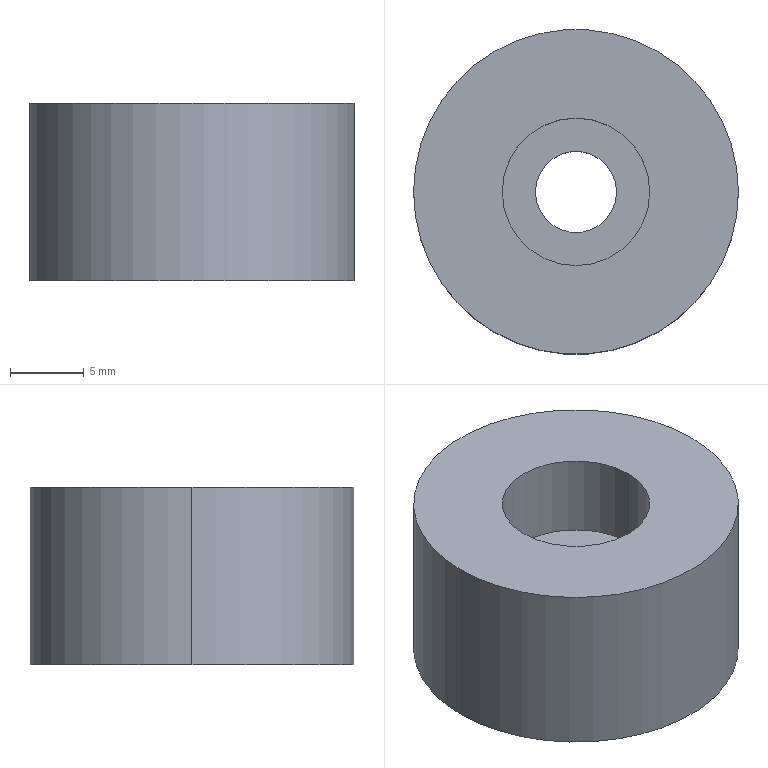Part | SolidWorks | features 3DProfileFeature 1, Extrusion 1, HoleWzd 1 | 1 solid | 9 faces | box 22 x 22 x 12 mm | volume 3964 mm3 | cylinder 6 | plane 3 | commonest cylinder face diameters 5.5 x2 10 x2 22 x2
STEP:
#1=CARTESIAN_POINT('',(-5.,0.,6.3));
#2=VERTEX_POINT('',#1);
#3=CARTESIAN_POINT('',(5.,0.,6.3));
#4=VERTEX_POINT('',#3);
#5=CARTESIAN_POINT('',(0.,0.,6.3));
#6=DIRECTION('',(0.,0.,1.));
#7=DIRECTION('',(1.,0.,0.));
#8=AXIS2_PLACEMENT_3D('',#5,#6,#7);
#9=CIRCLE('',#8,5.);
#10=EDGE_CURVE('',#2,#4,#9,.T.);
#11=ORIENTED_EDGE('',*,*,#10,.F.);
#12=CARTESIAN_POINT('',(-5.,0.,12.));
#13=VERTEX_POINT('',#12);
#14=CARTESIAN_POINT('',(-5.,0.,12.));
#15=DIRECTION('',(0.,0.,1.));
#16=VECTOR('',#15,1000.);
#17=LINE('',#14,#16);
#18=EDGE_CURVE('',#2,#13,#17,.T.);
#19=ORIENTED_EDGE('',*,*,#18,.T.);
#20=CARTESIAN_POINT('',(5.,0.,12.));
#21=VERTEX_POINT('',#20);
#22=CARTESIAN_POINT('',(0.,0.,12.));
#23=DIRECTION('',(0.,0.,1.));
#24=DIRECTION('',(1.,0.,0.));
#25=AXIS2_PLACEMENT_3D('',#22,#23,#24);
#26=CIRCLE('',#25,5.);
#27=EDGE_CURVE('',#13,#21,#26,.T.);
#28=ORIENTED_EDGE('',*,*,#27,.T.);
#29=CARTESIAN_POINT('',(5.,0.,12.));
#30=DIRECTION('',(0.,0.,1.));
#31=VECTOR('',#30,1000.);
#32=LINE('',#29,#31);
#33=EDGE_CURVE('',#4,#21,#32,.T.);
#34=ORIENTED_EDGE('',*,*,#33,.F.);
#35=EDGE_LOOP('',(#11,#19,#28,#34));
#36=FACE_OUTER_BOUND('',#35,.T.);
#37=CARTESIAN_POINT('',(0.,0.,12.));
#38=DIRECTION('',(0.,0.,1.));
#39=DIRECTION('',(1.,0.,0.));
#40=AXIS2_PLACEMENT_3D('',#37,#38,#39);
#41=CYLINDRICAL_SURFACE('',#40,5.);
#42=ADVANCED_FACE('',(#36),#41,.F.);
#43=CARTESIAN_POINT('',(-2.75,0.,0.));
#44=VERTEX_POINT('',#43);
#45=CARTESIAN_POINT('',(2.75,0.,0.));
#46=VERTEX_POINT('',#45);
#47=CARTESIAN_POINT('',(0.,0.,0.));
#48=DIRECTION('',(0.,0.,1.));
#49=DIRECTION('',(1.,0.,0.));
#50=AXIS2_PLACEMENT_3D('',#47,#48,#49);
#51=CIRCLE('',#50,2.75);
#52=EDGE_CURVE('',#44,#46,#51,.T.);
#53=ORIENTED_EDGE('',*,*,#52,.F.);
#54=CARTESIAN_POINT('',(-2.75,0.,6.3));
#55=VERTEX_POINT('',#54);
#56=CARTESIAN_POINT('',(-2.75,0.,12.));
#57=DIRECTION('',(0.,0.,1.));
#58=VECTOR('',#57,1000.);
#59=LINE('',#56,#58);
#60=EDGE_CURVE('',#44,#55,#59,.T.);
#61=ORIENTED_EDGE('',*,*,#60,.T.);
#62=CARTESIAN_POINT('',(2.75,0.,6.3));
#63=VERTEX_POINT('',#62);
#64=CARTESIAN_POINT('',(0.,0.,6.3));
#65=DIRECTION('',(0.,0.,1.));
#66=DIRECTION('',(1.,0.,0.));
#67=AXIS2_PLACEMENT_3D('',#64,#65,#66);
#68=CIRCLE('',#67,2.75);
#69=EDGE_CURVE('',#55,#63,#68,.T.);
#70=ORIENTED_EDGE('',*,*,#69,.T.);
#71=CARTESIAN_POINT('',(2.75,0.,12.));
#72=DIRECTION('',(0.,0.,1.));
#73=VECTOR('',#72,1000.);
#74=LINE('',#71,#73);
#75=EDGE_CURVE('',#46,#63,#74,.T.);
#76=ORIENTED_EDGE('',*,*,#75,.F.);
#77=EDGE_LOOP('',(#53,#61,#70,#76));
#78=FACE_OUTER_BOUND('',#77,.T.);
#79=CARTESIAN_POINT('',(0.,0.,12.));
#80=DIRECTION('',(0.,0.,1.));
#81=DIRECTION('',(1.,0.,0.));
#82=AXIS2_PLACEMENT_3D('',#79,#80,#81);
#83=CYLINDRICAL_SURFACE('',#82,2.75);
#84=ADVANCED_FACE('',(#78),#83,.F.);
#85=CARTESIAN_POINT('',(11.,0.,12.));
#86=VERTEX_POINT('',#85);
#87=CARTESIAN_POINT('',(-11.,0.,12.));
#88=VERTEX_POINT('',#87);
#89=CARTESIAN_POINT('',(0.,0.,12.));
#90=DIRECTION('',(0.,0.,1.));
#91=DIRECTION('',(1.,0.,0.));
#92=AXIS2_PLACEMENT_3D('',#89,#90,#91);
#93=CIRCLE('',#92,11.);
#94=EDGE_CURVE('',#86,#88,#93,.T.);
#95=ORIENTED_EDGE('',*,*,#94,.F.);
#96=CARTESIAN_POINT('',(11.,0.,0.));
#97=VERTEX_POINT('',#96);
#98=CARTESIAN_POINT('',(11.,0.,12.));
#99=DIRECTION('',(0.,0.,-1.));
#100=VECTOR('',#99,1000.);
#101=LINE('',#98,#100);
#102=EDGE_CURVE('',#86,#97,#101,.T.);
#103=ORIENTED_EDGE('',*,*,#102,.T.);
#104=CARTESIAN_POINT('',(-11.,0.,0.));
#105=VERTEX_POINT('',#104);
#106=CARTESIAN_POINT('',(0.,0.,0.));
#107=DIRECTION('',(0.,0.,1.));
#108=DIRECTION('',(1.,0.,0.));
#109=AXIS2_PLACEMENT_3D('',#106,#107,#108);
#110=CIRCLE('',#109,11.);
#111=EDGE_CURVE('',#97,#105,#110,.T.);
#112=ORIENTED_EDGE('',*,*,#111,.T.);
#113=CARTESIAN_POINT('',(-11.,0.,12.));
#114=DIRECTION('',(0.,0.,-1.));
#115=VECTOR('',#114,1000.);
#116=LINE('',#113,#115);
#117=EDGE_CURVE('',#88,#105,#116,.T.);
#118=ORIENTED_EDGE('',*,*,#117,.F.);
#119=EDGE_LOOP('',(#95,#103,#112,#118));
#120=FACE_OUTER_BOUND('',#119,.T.);
#121=CARTESIAN_POINT('',(0.,0.,12.));
#122=DIRECTION('',(0.,0.,-1.));
#123=DIRECTION('',(-1.,0.,0.));
#124=AXIS2_PLACEMENT_3D('',#121,#122,#123);
#125=CYLINDRICAL_SURFACE('',#124,11.);
#126=ADVANCED_FACE('',(#120),#125,.T.);
#127=ORIENTED_EDGE('',*,*,#102,.F.);
#128=CARTESIAN_POINT('',(0.,0.,12.));
#129=DIRECTION('',(0.,0.,1.));
#130=DIRECTION('',(1.,0.,0.));
#131=AXIS2_PLACEMENT_3D('',#128,#129,#130);
#132=CIRCLE('',#131,11.);
#133=EDGE_CURVE('',#88,#86,#132,.T.);
#134=ORIENTED_EDGE('',*,*,#133,.F.);
#135=ORIENTED_EDGE('',*,*,#117,.T.);
#136=CARTESIAN_POINT('',(0.,0.,0.));
#137=DIRECTION('',(0.,0.,1.));
#138=DIRECTION('',(1.,0.,0.));
#139=AXIS2_PLACEMENT_3D('',#136,#137,#138);
#140=CIRCLE('',#139,11.);
#141=EDGE_CURVE('',#105,#97,#140,.T.);
#142=ORIENTED_EDGE('',*,*,#141,.T.);
#143=EDGE_LOOP('',(#127,#134,#135,#142));
#144=FACE_OUTER_BOUND('',#143,.T.);
#145=CARTESIAN_POINT('',(0.,0.,12.));
#146=DIRECTION('',(0.,0.,-1.));
#147=DIRECTION('',(-1.,0.,0.));
#148=AXIS2_PLACEMENT_3D('',#145,#146,#147);
#149=CYLINDRICAL_SURFACE('',#148,11.);
#150=ADVANCED_FACE('',(#144),#149,.T.);
#151=CARTESIAN_POINT('',(0.,0.,12.));
#152=DIRECTION('',(0.,0.,1.));
#153=DIRECTION('',(1.,0.,0.));
#154=AXIS2_PLACEMENT_3D('',#151,#152,#153);
#155=CIRCLE('',#154,5.);
#156=EDGE_CURVE('',#21,#13,#155,.T.);
#157=ORIENTED_EDGE('',*,*,#156,.F.);
#158=ORIENTED_EDGE('',*,*,#27,.F.);
#159=EDGE_LOOP('',(#157,#158));
#160=FACE_BOUND('',#159,.T.);
#161=ORIENTED_EDGE('',*,*,#133,.T.);
#162=ORIENTED_EDGE('',*,*,#94,.T.);
#163=EDGE_LOOP('',(#161,#162));
#164=FACE_OUTER_BOUND('',#163,.T.);
#165=CARTESIAN_POINT('',(0.,0.,12.));
#166=DIRECTION('',(0.,0.,1.));
#167=DIRECTION('',(1.,0.,0.));
#168=AXIS2_PLACEMENT_3D('',#165,#166,#167);
#169=PLANE('',#168);
#170=ADVANCED_FACE('',(#160,#164),#169,.T.);
#171=CARTESIAN_POINT('',(0.,0.,0.));
#172=DIRECTION('',(0.,0.,1.));
#173=DIRECTION('',(1.,0.,0.));
#174=AXIS2_PLACEMENT_3D('',#171,#172,#173);
#175=CIRCLE('',#174,2.75);
#176=EDGE_CURVE('',#46,#44,#175,.T.);
#177=ORIENTED_EDGE('',*,*,#176,.T.);
#178=ORIENTED_EDGE('',*,*,#52,.T.);
#179=EDGE_LOOP('',(#177,#178));
#180=FACE_BOUND('',#179,.T.);
#181=ORIENTED_EDGE('',*,*,#141,.F.);
#182=ORIENTED_EDGE('',*,*,#111,.F.);
#183=EDGE_LOOP('',(#181,#182));
#184=FACE_OUTER_BOUND('',#183,.T.);
#185=CARTESIAN_POINT('',(0.,0.,0.));
#186=DIRECTION('',(0.,0.,1.));
#187=DIRECTION('',(1.,0.,0.));
#188=AXIS2_PLACEMENT_3D('',#185,#186,#187);
#189=PLANE('',#188);
#190=ADVANCED_FACE('',(#180,#184),#189,.F.);
#191=ORIENTED_EDGE('',*,*,#60,.F.);
#192=ORIENTED_EDGE('',*,*,#176,.F.);
#193=ORIENTED_EDGE('',*,*,#75,.T.);
#194=CARTESIAN_POINT('',(0.,0.,6.3));
#195=DIRECTION('',(0.,0.,1.));
#196=DIRECTION('',(1.,0.,0.));
#197=AXIS2_PLACEMENT_3D('',#194,#195,#196);
#198=CIRCLE('',#197,2.75);
#199=EDGE_CURVE('',#63,#55,#198,.T.);
#200=ORIENTED_EDGE('',*,*,#199,.T.);
#201=EDGE_LOOP('',(#191,#192,#193,#200));
#202=FACE_OUTER_BOUND('',#201,.T.);
#203=CARTESIAN_POINT('',(0.,0.,12.));
#204=DIRECTION('',(0.,0.,1.));
#205=DIRECTION('',(1.,0.,0.));
#206=AXIS2_PLACEMENT_3D('',#203,#204,#205);
#207=CYLINDRICAL_SURFACE('',#206,2.75);
#208=ADVANCED_FACE('',(#202),#207,.F.);
#209=ORIENTED_EDGE('',*,*,#199,.F.);
#210=ORIENTED_EDGE('',*,*,#69,.F.);
#211=EDGE_LOOP('',(#209,#210));
#212=FACE_BOUND('',#211,.T.);
#213=CARTESIAN_POINT('',(0.,0.,6.3));
#214=DIRECTION('',(0.,0.,1.));
#215=DIRECTION('',(1.,0.,0.));
#216=AXIS2_PLACEMENT_3D('',#213,#214,#215);
#217=CIRCLE('',#216,5.);
#218=EDGE_CURVE('',#4,#2,#217,.T.);
#219=ORIENTED_EDGE('',*,*,#218,.T.);
#220=ORIENTED_EDGE('',*,*,#10,.T.);
#221=EDGE_LOOP('',(#219,#220));
#222=FACE_OUTER_BOUND('',#221,.T.);
#223=CARTESIAN_POINT('',(2.75,0.,6.3));
#224=DIRECTION('',(0.,0.,-1.));
#225=DIRECTION('',(-1.,0.,0.));
#226=AXIS2_PLACEMENT_3D('',#223,#224,#225);
#227=PLANE('',#226);
#228=ADVANCED_FACE('',(#212,#222),#227,.F.);
#229=ORIENTED_EDGE('',*,*,#18,.F.);
#230=ORIENTED_EDGE('',*,*,#218,.F.);
#231=ORIENTED_EDGE('',*,*,#33,.T.);
#232=ORIENTED_EDGE('',*,*,#156,.T.);
#233=EDGE_LOOP('',(#229,#230,#231,#232));
#234=FACE_OUTER_BOUND('',#233,.T.);
#235=CARTESIAN_POINT('',(0.,0.,12.));
#236=DIRECTION('',(0.,0.,1.));
#237=DIRECTION('',(1.,0.,0.));
#238=AXIS2_PLACEMENT_3D('',#235,#236,#237);
#239=CYLINDRICAL_SURFACE('',#238,5.);
#240=ADVANCED_FACE('',(#234),#239,.F.);
#241=CLOSED_SHELL('',(#42,#84,#126,#150,#170,#190,#208,#228,#240));
#242=MANIFOLD_SOLID_BREP('',#241);
#243=CARTESIAN_POINT('',(0.,0.,0.));
#244=DIRECTION('',(0.,0.,1.));
#245=DIRECTION('',(1.,0.,0.));
#246=AXIS2_PLACEMENT_3D('',#243,#244,#245);
#247=(LENGTH_UNIT()NAMED_UNIT(*)SI_UNIT(.MILLI.,.METRE.));
#248=UNCERTAINTY_MEASURE_WITH_UNIT(LENGTH_MEASURE(0.00001),#247,'','');
#249=(NAMED_UNIT(*)PLANE_ANGLE_UNIT()SI_UNIT($,.RADIAN.));
#250=(NAMED_UNIT(*)SI_UNIT($,.STERADIAN.)SOLID_ANGLE_UNIT());
#251=(GEOMETRIC_REPRESENTATION_CONTEXT(3)GLOBAL_UNCERTAINTY_ASSIGNED_CONTEXT((#248))GLOBAL_UNIT_ASSIGNED_CONTEXT((#247,#249,#250))REPRESENTATION_CONTEXT('',''));
#252=ADVANCED_BREP_SHAPE_REPRESENTATION('',(#242,#246),#251);